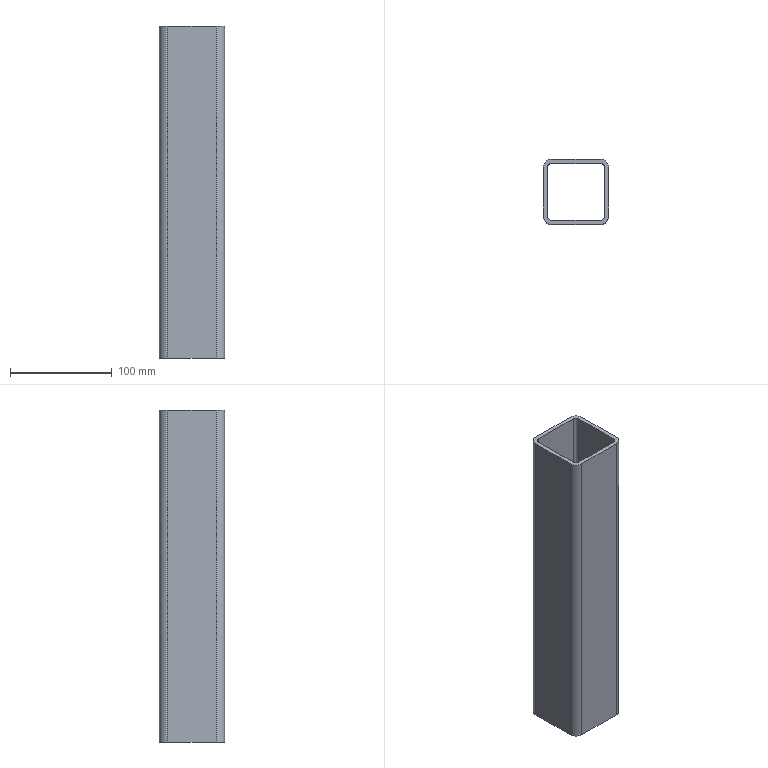Part | SolidWorks | features Extrusion 1 | 1 solid | 18 faces | box 64 x 64 x 326 mm | volume 299528 mm3 | plane 10 | cylinder 8 | commonest cylinder face diameters 8 x4 16 x4
STEP:
#1=CARTESIAN_POINT('',(-24.,32.,163.));
#2=VERTEX_POINT('',#1);
#3=CARTESIAN_POINT('',(-32.,24.,163.));
#4=VERTEX_POINT('',#3);
#5=CARTESIAN_POINT('',(-24.,24.,163.));
#6=DIRECTION('',(0.,0.,1.));
#7=DIRECTION('',(1.,0.,0.));
#8=AXIS2_PLACEMENT_3D('',#5,#6,#7);
#9=CIRCLE('',#8,8.);
#10=EDGE_CURVE('',#2,#4,#9,.T.);
#11=ORIENTED_EDGE('',*,*,#10,.T.);
#12=CARTESIAN_POINT('',(-32.,-24.,163.));
#13=VERTEX_POINT('',#12);
#14=CARTESIAN_POINT('',(-32.,24.,163.));
#15=DIRECTION('',(0.,-1.,0.));
#16=VECTOR('',#15,1000.);
#17=LINE('',#14,#16);
#18=EDGE_CURVE('',#4,#13,#17,.T.);
#19=ORIENTED_EDGE('',*,*,#18,.T.);
#20=CARTESIAN_POINT('',(-24.,-32.,163.));
#21=VERTEX_POINT('',#20);
#22=CARTESIAN_POINT('',(-24.,-24.,163.));
#23=DIRECTION('',(0.,0.,1.));
#24=DIRECTION('',(-1.,0.,0.));
#25=AXIS2_PLACEMENT_3D('',#22,#23,#24);
#26=CIRCLE('',#25,8.);
#27=EDGE_CURVE('',#13,#21,#26,.T.);
#28=ORIENTED_EDGE('',*,*,#27,.T.);
#29=CARTESIAN_POINT('',(24.,-32.,163.));
#30=VERTEX_POINT('',#29);
#31=CARTESIAN_POINT('',(24.,-32.,163.));
#32=DIRECTION('',(1.,0.,0.));
#33=VECTOR('',#32,1000.);
#34=LINE('',#31,#33);
#35=EDGE_CURVE('',#21,#30,#34,.T.);
#36=ORIENTED_EDGE('',*,*,#35,.T.);
#37=CARTESIAN_POINT('',(32.,-24.,163.));
#38=VERTEX_POINT('',#37);
#39=CARTESIAN_POINT('',(24.,-24.,163.));
#40=DIRECTION('',(0.,0.,1.));
#41=DIRECTION('',(1.,0.,0.));
#42=AXIS2_PLACEMENT_3D('',#39,#40,#41);
#43=CIRCLE('',#42,8.);
#44=EDGE_CURVE('',#30,#38,#43,.T.);
#45=ORIENTED_EDGE('',*,*,#44,.T.);
#46=CARTESIAN_POINT('',(32.,24.,163.));
#47=VERTEX_POINT('',#46);
#48=CARTESIAN_POINT('',(32.,-24.,163.));
#49=DIRECTION('',(0.,1.,0.));
#50=VECTOR('',#49,1000.);
#51=LINE('',#48,#50);
#52=EDGE_CURVE('',#38,#47,#51,.T.);
#53=ORIENTED_EDGE('',*,*,#52,.T.);
#54=CARTESIAN_POINT('',(24.,32.,163.));
#55=VERTEX_POINT('',#54);
#56=CARTESIAN_POINT('',(24.,24.,163.));
#57=DIRECTION('',(0.,0.,1.));
#58=DIRECTION('',(-1.,0.,0.));
#59=AXIS2_PLACEMENT_3D('',#56,#57,#58);
#60=CIRCLE('',#59,8.);
#61=EDGE_CURVE('',#47,#55,#60,.T.);
#62=ORIENTED_EDGE('',*,*,#61,.T.);
#63=CARTESIAN_POINT('',(0.,32.,163.));
#64=DIRECTION('',(-1.,0.,0.));
#65=VECTOR('',#64,1000.);
#66=LINE('',#63,#65);
#67=EDGE_CURVE('',#55,#2,#66,.T.);
#68=ORIENTED_EDGE('',*,*,#67,.T.);
#69=EDGE_LOOP('',(#11,#19,#28,#36,#45,#53,#62,#68));
#70=FACE_OUTER_BOUND('',#69,.T.);
#71=CARTESIAN_POINT('',(-28.,24.,163.));
#72=VERTEX_POINT('',#71);
#73=CARTESIAN_POINT('',(-28.,-24.,163.));
#74=VERTEX_POINT('',#73);
#75=CARTESIAN_POINT('',(-28.,24.,163.));
#76=DIRECTION('',(0.,-1.,0.));
#77=VECTOR('',#76,1000.);
#78=LINE('',#75,#77);
#79=EDGE_CURVE('',#72,#74,#78,.T.);
#80=ORIENTED_EDGE('',*,*,#79,.F.);
#81=CARTESIAN_POINT('',(-24.,28.,163.));
#82=VERTEX_POINT('',#81);
#83=CARTESIAN_POINT('',(-24.,24.,163.));
#84=DIRECTION('',(0.,0.,1.));
#85=DIRECTION('',(1.,0.,0.));
#86=AXIS2_PLACEMENT_3D('',#83,#84,#85);
#87=CIRCLE('',#86,4.);
#88=EDGE_CURVE('',#82,#72,#87,.T.);
#89=ORIENTED_EDGE('',*,*,#88,.F.);
#90=CARTESIAN_POINT('',(24.,28.,163.));
#91=VERTEX_POINT('',#90);
#92=CARTESIAN_POINT('',(0.,28.,163.));
#93=DIRECTION('',(-1.,0.,0.));
#94=VECTOR('',#93,1000.);
#95=LINE('',#92,#94);
#96=EDGE_CURVE('',#91,#82,#95,.T.);
#97=ORIENTED_EDGE('',*,*,#96,.F.);
#98=CARTESIAN_POINT('',(28.,24.,163.));
#99=VERTEX_POINT('',#98);
#100=CARTESIAN_POINT('',(24.,24.,163.));
#101=DIRECTION('',(0.,0.,1.));
#102=DIRECTION('',(-1.,0.,0.));
#103=AXIS2_PLACEMENT_3D('',#100,#101,#102);
#104=CIRCLE('',#103,4.);
#105=EDGE_CURVE('',#99,#91,#104,.T.);
#106=ORIENTED_EDGE('',*,*,#105,.F.);
#107=CARTESIAN_POINT('',(28.,-24.,163.));
#108=VERTEX_POINT('',#107);
#109=CARTESIAN_POINT('',(28.,-24.,163.));
#110=DIRECTION('',(0.,1.,0.));
#111=VECTOR('',#110,1000.);
#112=LINE('',#109,#111);
#113=EDGE_CURVE('',#108,#99,#112,.T.);
#114=ORIENTED_EDGE('',*,*,#113,.F.);
#115=CARTESIAN_POINT('',(24.,-28.,163.));
#116=VERTEX_POINT('',#115);
#117=CARTESIAN_POINT('',(24.,-24.,163.));
#118=DIRECTION('',(0.,0.,1.));
#119=DIRECTION('',(1.,0.,0.));
#120=AXIS2_PLACEMENT_3D('',#117,#118,#119);
#121=CIRCLE('',#120,4.);
#122=EDGE_CURVE('',#116,#108,#121,.T.);
#123=ORIENTED_EDGE('',*,*,#122,.F.);
#124=CARTESIAN_POINT('',(-24.,-28.,163.));
#125=VERTEX_POINT('',#124);
#126=CARTESIAN_POINT('',(24.,-28.,163.));
#127=DIRECTION('',(1.,0.,0.));
#128=VECTOR('',#127,1000.);
#129=LINE('',#126,#128);
#130=EDGE_CURVE('',#125,#116,#129,.T.);
#131=ORIENTED_EDGE('',*,*,#130,.F.);
#132=CARTESIAN_POINT('',(-24.,-24.,163.));
#133=DIRECTION('',(0.,0.,1.));
#134=DIRECTION('',(-1.,0.,0.));
#135=AXIS2_PLACEMENT_3D('',#132,#133,#134);
#136=CIRCLE('',#135,4.);
#137=EDGE_CURVE('',#74,#125,#136,.T.);
#138=ORIENTED_EDGE('',*,*,#137,.F.);
#139=EDGE_LOOP('',(#80,#89,#97,#106,#114,#123,#131,#138));
#140=FACE_BOUND('',#139,.T.);
#141=CARTESIAN_POINT('',(-24.,24.,163.));
#142=DIRECTION('',(0.,0.,1.));
#143=DIRECTION('',(1.,0.,0.));
#144=AXIS2_PLACEMENT_3D('',#141,#142,#143);
#145=PLANE('',#144);
#146=ADVANCED_FACE('',(#70,#140),#145,.T.);
#147=CARTESIAN_POINT('',(-24.,32.,-163.));
#148=VERTEX_POINT('',#147);
#149=CARTESIAN_POINT('',(-32.,24.,-163.));
#150=VERTEX_POINT('',#149);
#151=CARTESIAN_POINT('',(-24.,24.,-163.));
#152=DIRECTION('',(0.,0.,1.));
#153=DIRECTION('',(1.,0.,0.));
#154=AXIS2_PLACEMENT_3D('',#151,#152,#153);
#155=CIRCLE('',#154,8.);
#156=EDGE_CURVE('',#148,#150,#155,.T.);
#157=ORIENTED_EDGE('',*,*,#156,.F.);
#158=CARTESIAN_POINT('',(24.,32.,-163.));
#159=VERTEX_POINT('',#158);
#160=CARTESIAN_POINT('',(0.,32.,-163.));
#161=DIRECTION('',(-1.,0.,0.));
#162=VECTOR('',#161,1000.);
#163=LINE('',#160,#162);
#164=EDGE_CURVE('',#159,#148,#163,.T.);
#165=ORIENTED_EDGE('',*,*,#164,.F.);
#166=CARTESIAN_POINT('',(32.,24.,-163.));
#167=VERTEX_POINT('',#166);
#168=CARTESIAN_POINT('',(24.,24.,-163.));
#169=DIRECTION('',(0.,0.,1.));
#170=DIRECTION('',(-1.,0.,0.));
#171=AXIS2_PLACEMENT_3D('',#168,#169,#170);
#172=CIRCLE('',#171,8.);
#173=EDGE_CURVE('',#167,#159,#172,.T.);
#174=ORIENTED_EDGE('',*,*,#173,.F.);
#175=CARTESIAN_POINT('',(32.,-24.,-163.));
#176=VERTEX_POINT('',#175);
#177=CARTESIAN_POINT('',(32.,24.,-163.));
#178=DIRECTION('',(0.,1.,0.));
#179=VECTOR('',#178,1000.);
#180=LINE('',#177,#179);
#181=EDGE_CURVE('',#176,#167,#180,.T.);
#182=ORIENTED_EDGE('',*,*,#181,.F.);
#183=CARTESIAN_POINT('',(24.,-32.,-163.));
#184=VERTEX_POINT('',#183);
#185=CARTESIAN_POINT('',(24.,-24.,-163.));
#186=DIRECTION('',(0.,0.,1.));
#187=DIRECTION('',(1.,0.,0.));
#188=AXIS2_PLACEMENT_3D('',#185,#186,#187);
#189=CIRCLE('',#188,8.);
#190=EDGE_CURVE('',#184,#176,#189,.T.);
#191=ORIENTED_EDGE('',*,*,#190,.F.);
#192=CARTESIAN_POINT('',(-24.,-32.,-163.));
#193=VERTEX_POINT('',#192);
#194=CARTESIAN_POINT('',(24.,-32.,-163.));
#195=DIRECTION('',(1.,0.,0.));
#196=VECTOR('',#195,1000.);
#197=LINE('',#194,#196);
#198=EDGE_CURVE('',#193,#184,#197,.T.);
#199=ORIENTED_EDGE('',*,*,#198,.F.);
#200=CARTESIAN_POINT('',(-32.,-24.,-163.));
#201=VERTEX_POINT('',#200);
#202=CARTESIAN_POINT('',(-24.,-24.,-163.));
#203=DIRECTION('',(0.,0.,1.));
#204=DIRECTION('',(-1.,0.,0.));
#205=AXIS2_PLACEMENT_3D('',#202,#203,#204);
#206=CIRCLE('',#205,8.);
#207=EDGE_CURVE('',#201,#193,#206,.T.);
#208=ORIENTED_EDGE('',*,*,#207,.F.);
#209=CARTESIAN_POINT('',(-32.,-24.,-163.));
#210=DIRECTION('',(0.,-1.,0.));
#211=VECTOR('',#210,1000.);
#212=LINE('',#209,#211);
#213=EDGE_CURVE('',#150,#201,#212,.T.);
#214=ORIENTED_EDGE('',*,*,#213,.F.);
#215=EDGE_LOOP('',(#157,#165,#174,#182,#191,#199,#208,#214));
#216=FACE_OUTER_BOUND('',#215,.T.);
#217=CARTESIAN_POINT('',(-24.,28.,-163.));
#218=VERTEX_POINT('',#217);
#219=CARTESIAN_POINT('',(-28.,24.,-163.));
#220=VERTEX_POINT('',#219);
#221=CARTESIAN_POINT('',(-24.,24.,-163.));
#222=DIRECTION('',(0.,0.,1.));
#223=DIRECTION('',(1.,0.,0.));
#224=AXIS2_PLACEMENT_3D('',#221,#222,#223);
#225=CIRCLE('',#224,4.);
#226=EDGE_CURVE('',#218,#220,#225,.T.);
#227=ORIENTED_EDGE('',*,*,#226,.T.);
#228=CARTESIAN_POINT('',(-28.,-24.,-163.));
#229=VERTEX_POINT('',#228);
#230=CARTESIAN_POINT('',(-28.,-24.,-163.));
#231=DIRECTION('',(0.,-1.,0.));
#232=VECTOR('',#231,1000.);
#233=LINE('',#230,#232);
#234=EDGE_CURVE('',#220,#229,#233,.T.);
#235=ORIENTED_EDGE('',*,*,#234,.T.);
#236=CARTESIAN_POINT('',(-24.,-28.,-163.));
#237=VERTEX_POINT('',#236);
#238=CARTESIAN_POINT('',(-24.,-24.,-163.));
#239=DIRECTION('',(0.,0.,1.));
#240=DIRECTION('',(-1.,0.,0.));
#241=AXIS2_PLACEMENT_3D('',#238,#239,#240);
#242=CIRCLE('',#241,4.);
#243=EDGE_CURVE('',#229,#237,#242,.T.);
#244=ORIENTED_EDGE('',*,*,#243,.T.);
#245=CARTESIAN_POINT('',(24.,-28.,-163.));
#246=VERTEX_POINT('',#245);
#247=CARTESIAN_POINT('',(24.,-28.,-163.));
#248=DIRECTION('',(1.,0.,0.));
#249=VECTOR('',#248,1000.);
#250=LINE('',#247,#249);
#251=EDGE_CURVE('',#237,#246,#250,.T.);
#252=ORIENTED_EDGE('',*,*,#251,.T.);
#253=CARTESIAN_POINT('',(28.,-24.,-163.));
#254=VERTEX_POINT('',#253);
#255=CARTESIAN_POINT('',(24.,-24.,-163.));
#256=DIRECTION('',(0.,0.,1.));
#257=DIRECTION('',(1.,0.,0.));
#258=AXIS2_PLACEMENT_3D('',#255,#256,#257);
#259=CIRCLE('',#258,4.);
#260=EDGE_CURVE('',#246,#254,#259,.T.);
#261=ORIENTED_EDGE('',*,*,#260,.T.);
#262=CARTESIAN_POINT('',(28.,24.,-163.));
#263=VERTEX_POINT('',#262);
#264=CARTESIAN_POINT('',(28.,24.,-163.));
#265=DIRECTION('',(0.,1.,0.));
#266=VECTOR('',#265,1000.);
#267=LINE('',#264,#266);
#268=EDGE_CURVE('',#254,#263,#267,.T.);
#269=ORIENTED_EDGE('',*,*,#268,.T.);
#270=CARTESIAN_POINT('',(24.,28.,-163.));
#271=VERTEX_POINT('',#270);
#272=CARTESIAN_POINT('',(24.,24.,-163.));
#273=DIRECTION('',(0.,0.,1.));
#274=DIRECTION('',(-1.,0.,0.));
#275=AXIS2_PLACEMENT_3D('',#272,#273,#274);
#276=CIRCLE('',#275,4.);
#277=EDGE_CURVE('',#263,#271,#276,.T.);
#278=ORIENTED_EDGE('',*,*,#277,.T.);
#279=CARTESIAN_POINT('',(0.,28.,-163.));
#280=DIRECTION('',(-1.,0.,0.));
#281=VECTOR('',#280,1000.);
#282=LINE('',#279,#281);
#283=EDGE_CURVE('',#271,#218,#282,.T.);
#284=ORIENTED_EDGE('',*,*,#283,.T.);
#285=EDGE_LOOP('',(#227,#235,#244,#252,#261,#269,#278,#284));
#286=FACE_BOUND('',#285,.T.);
#287=CARTESIAN_POINT('',(-24.,24.,-163.));
#288=DIRECTION('',(0.,0.,1.));
#289=DIRECTION('',(1.,0.,0.));
#290=AXIS2_PLACEMENT_3D('',#287,#288,#289);
#291=PLANE('',#290);
#292=ADVANCED_FACE('',(#216,#286),#291,.F.);
#293=ORIENTED_EDGE('',*,*,#156,.T.);
#294=CARTESIAN_POINT('',(-32.,24.,163.));
#295=DIRECTION('',(0.,0.,-1.));
#296=VECTOR('',#295,1000.);
#297=LINE('',#294,#296);
#298=EDGE_CURVE('',#4,#150,#297,.T.);
#299=ORIENTED_EDGE('',*,*,#298,.F.);
#300=ORIENTED_EDGE('',*,*,#10,.F.);
#301=CARTESIAN_POINT('',(-24.,32.,163.));
#302=DIRECTION('',(0.,0.,-1.));
#303=VECTOR('',#302,1000.);
#304=LINE('',#301,#303);
#305=EDGE_CURVE('',#2,#148,#304,.T.);
#306=ORIENTED_EDGE('',*,*,#305,.T.);
#307=EDGE_LOOP('',(#293,#299,#300,#306));
#308=FACE_OUTER_BOUND('',#307,.T.);
#309=CARTESIAN_POINT('',(-24.,24.,163.));
#310=DIRECTION('',(0.,0.,-1.));
#311=DIRECTION('',(-1.,0.,0.));
#312=AXIS2_PLACEMENT_3D('',#309,#310,#311);
#313=CYLINDRICAL_SURFACE('',#312,8.);
#314=ADVANCED_FACE('',(#308),#313,.T.);
#315=ORIENTED_EDGE('',*,*,#213,.T.);
#316=CARTESIAN_POINT('',(-32.,-24.,163.));
#317=DIRECTION('',(0.,0.,-1.));
#318=VECTOR('',#317,1000.);
#319=LINE('',#316,#318);
#320=EDGE_CURVE('',#13,#201,#319,.T.);
#321=ORIENTED_EDGE('',*,*,#320,.F.);
#322=ORIENTED_EDGE('',*,*,#18,.F.);
#323=ORIENTED_EDGE('',*,*,#298,.T.);
#324=EDGE_LOOP('',(#315,#321,#322,#323));
#325=FACE_OUTER_BOUND('',#324,.T.);
#326=CARTESIAN_POINT('',(-32.,-24.,163.));
#327=DIRECTION('',(1.,0.,0.));
#328=DIRECTION('',(0.,0.,-1.));
#329=AXIS2_PLACEMENT_3D('',#326,#327,#328);
#330=PLANE('',#329);
#331=ADVANCED_FACE('',(#325),#330,.F.);
#332=ORIENTED_EDGE('',*,*,#207,.T.);
#333=CARTESIAN_POINT('',(-24.,-32.,163.));
#334=DIRECTION('',(0.,0.,-1.));
#335=VECTOR('',#334,1000.);
#336=LINE('',#333,#335);
#337=EDGE_CURVE('',#21,#193,#336,.T.);
#338=ORIENTED_EDGE('',*,*,#337,.F.);
#339=ORIENTED_EDGE('',*,*,#27,.F.);
#340=ORIENTED_EDGE('',*,*,#320,.T.);
#341=EDGE_LOOP('',(#332,#338,#339,#340));
#342=FACE_OUTER_BOUND('',#341,.T.);
#343=CARTESIAN_POINT('',(-24.,-24.,163.));
#344=DIRECTION('',(0.,0.,-1.));
#345=DIRECTION('',(-1.,0.,0.));
#346=AXIS2_PLACEMENT_3D('',#343,#344,#345);
#347=CYLINDRICAL_SURFACE('',#346,8.);
#348=ADVANCED_FACE('',(#342),#347,.T.);
#349=ORIENTED_EDGE('',*,*,#198,.T.);
#350=CARTESIAN_POINT('',(24.,-32.,163.));
#351=DIRECTION('',(0.,0.,-1.));
#352=VECTOR('',#351,1000.);
#353=LINE('',#350,#352);
#354=EDGE_CURVE('',#30,#184,#353,.T.);
#355=ORIENTED_EDGE('',*,*,#354,.F.);
#356=ORIENTED_EDGE('',*,*,#35,.F.);
#357=ORIENTED_EDGE('',*,*,#337,.T.);
#358=EDGE_LOOP('',(#349,#355,#356,#357));
#359=FACE_OUTER_BOUND('',#358,.T.);
#360=CARTESIAN_POINT('',(24.,-32.,163.));
#361=DIRECTION('',(0.,1.,0.));
#362=DIRECTION('',(-1.,0.,0.));
#363=AXIS2_PLACEMENT_3D('',#360,#361,#362);
#364=PLANE('',#363);
#365=ADVANCED_FACE('',(#359),#364,.F.);
#366=ORIENTED_EDGE('',*,*,#190,.T.);
#367=CARTESIAN_POINT('',(32.,-24.,163.));
#368=DIRECTION('',(0.,0.,-1.));
#369=VECTOR('',#368,1000.);
#370=LINE('',#367,#369);
#371=EDGE_CURVE('',#38,#176,#370,.T.);
#372=ORIENTED_EDGE('',*,*,#371,.F.);
#373=ORIENTED_EDGE('',*,*,#44,.F.);
#374=ORIENTED_EDGE('',*,*,#354,.T.);
#375=EDGE_LOOP('',(#366,#372,#373,#374));
#376=FACE_OUTER_BOUND('',#375,.T.);
#377=CARTESIAN_POINT('',(24.,-24.,163.));
#378=DIRECTION('',(0.,0.,-1.));
#379=DIRECTION('',(-1.,0.,0.));
#380=AXIS2_PLACEMENT_3D('',#377,#378,#379);
#381=CYLINDRICAL_SURFACE('',#380,8.);
#382=ADVANCED_FACE('',(#376),#381,.T.);
#383=ORIENTED_EDGE('',*,*,#181,.T.);
#384=CARTESIAN_POINT('',(32.,24.,163.));
#385=DIRECTION('',(0.,0.,-1.));
#386=VECTOR('',#385,1000.);
#387=LINE('',#384,#386);
#388=EDGE_CURVE('',#47,#167,#387,.T.);
#389=ORIENTED_EDGE('',*,*,#388,.F.);
#390=ORIENTED_EDGE('',*,*,#52,.F.);
#391=ORIENTED_EDGE('',*,*,#371,.T.);
#392=EDGE_LOOP('',(#383,#389,#390,#391));
#393=FACE_OUTER_BOUND('',#392,.T.);
#394=CARTESIAN_POINT('',(32.,24.,163.));
#395=DIRECTION('',(-1.,0.,0.));
#396=DIRECTION('',(0.,0.,1.));
#397=AXIS2_PLACEMENT_3D('',#394,#395,#396);
#398=PLANE('',#397);
#399=ADVANCED_FACE('',(#393),#398,.F.);
#400=ORIENTED_EDGE('',*,*,#173,.T.);
#401=CARTESIAN_POINT('',(24.,32.,163.));
#402=DIRECTION('',(0.,0.,-1.));
#403=VECTOR('',#402,1000.);
#404=LINE('',#401,#403);
#405=EDGE_CURVE('',#55,#159,#404,.T.);
#406=ORIENTED_EDGE('',*,*,#405,.F.);
#407=ORIENTED_EDGE('',*,*,#61,.F.);
#408=ORIENTED_EDGE('',*,*,#388,.T.);
#409=EDGE_LOOP('',(#400,#406,#407,#408));
#410=FACE_OUTER_BOUND('',#409,.T.);
#411=CARTESIAN_POINT('',(24.,24.,163.));
#412=DIRECTION('',(0.,0.,-1.));
#413=DIRECTION('',(-1.,0.,0.));
#414=AXIS2_PLACEMENT_3D('',#411,#412,#413);
#415=CYLINDRICAL_SURFACE('',#414,8.);
#416=ADVANCED_FACE('',(#410),#415,.T.);
#417=ORIENTED_EDGE('',*,*,#164,.T.);
#418=ORIENTED_EDGE('',*,*,#305,.F.);
#419=ORIENTED_EDGE('',*,*,#67,.F.);
#420=ORIENTED_EDGE('',*,*,#405,.T.);
#421=EDGE_LOOP('',(#417,#418,#419,#420));
#422=FACE_OUTER_BOUND('',#421,.T.);
#423=CARTESIAN_POINT('',(0.,32.,163.));
#424=DIRECTION('',(0.,-1.,0.));
#425=DIRECTION('',(0.,0.,-1.));
#426=AXIS2_PLACEMENT_3D('',#423,#424,#425);
#427=PLANE('',#426);
#428=ADVANCED_FACE('',(#422),#427,.F.);
#429=ORIENTED_EDGE('',*,*,#226,.F.);
#430=CARTESIAN_POINT('',(-24.,28.,163.));
#431=DIRECTION('',(0.,0.,-1.));
#432=VECTOR('',#431,1000.);
#433=LINE('',#430,#432);
#434=EDGE_CURVE('',#82,#218,#433,.T.);
#435=ORIENTED_EDGE('',*,*,#434,.F.);
#436=ORIENTED_EDGE('',*,*,#88,.T.);
#437=CARTESIAN_POINT('',(-28.,24.,163.));
#438=DIRECTION('',(0.,0.,-1.));
#439=VECTOR('',#438,1000.);
#440=LINE('',#437,#439);
#441=EDGE_CURVE('',#72,#220,#440,.T.);
#442=ORIENTED_EDGE('',*,*,#441,.T.);
#443=EDGE_LOOP('',(#429,#435,#436,#442));
#444=FACE_OUTER_BOUND('',#443,.T.);
#445=CARTESIAN_POINT('',(-24.,24.,163.));
#446=DIRECTION('',(0.,0.,-1.));
#447=DIRECTION('',(-1.,0.,0.));
#448=AXIS2_PLACEMENT_3D('',#445,#446,#447);
#449=CYLINDRICAL_SURFACE('',#448,4.);
#450=ADVANCED_FACE('',(#444),#449,.F.);
#451=ORIENTED_EDGE('',*,*,#234,.F.);
#452=ORIENTED_EDGE('',*,*,#441,.F.);
#453=ORIENTED_EDGE('',*,*,#79,.T.);
#454=CARTESIAN_POINT('',(-28.,-24.,163.));
#455=DIRECTION('',(0.,0.,-1.));
#456=VECTOR('',#455,1000.);
#457=LINE('',#454,#456);
#458=EDGE_CURVE('',#74,#229,#457,.T.);
#459=ORIENTED_EDGE('',*,*,#458,.T.);
#460=EDGE_LOOP('',(#451,#452,#453,#459));
#461=FACE_OUTER_BOUND('',#460,.T.);
#462=CARTESIAN_POINT('',(-28.,-24.,163.));
#463=DIRECTION('',(1.,0.,0.));
#464=DIRECTION('',(0.,1.,0.));
#465=AXIS2_PLACEMENT_3D('',#462,#463,#464);
#466=PLANE('',#465);
#467=ADVANCED_FACE('',(#461),#466,.T.);
#468=ORIENTED_EDGE('',*,*,#243,.F.);
#469=ORIENTED_EDGE('',*,*,#458,.F.);
#470=ORIENTED_EDGE('',*,*,#137,.T.);
#471=CARTESIAN_POINT('',(-24.,-28.,163.));
#472=DIRECTION('',(0.,0.,-1.));
#473=VECTOR('',#472,1000.);
#474=LINE('',#471,#473);
#475=EDGE_CURVE('',#125,#237,#474,.T.);
#476=ORIENTED_EDGE('',*,*,#475,.T.);
#477=EDGE_LOOP('',(#468,#469,#470,#476));
#478=FACE_OUTER_BOUND('',#477,.T.);
#479=CARTESIAN_POINT('',(-24.,-24.,163.));
#480=DIRECTION('',(0.,0.,-1.));
#481=DIRECTION('',(-1.,0.,0.));
#482=AXIS2_PLACEMENT_3D('',#479,#480,#481);
#483=CYLINDRICAL_SURFACE('',#482,4.);
#484=ADVANCED_FACE('',(#478),#483,.F.);
#485=ORIENTED_EDGE('',*,*,#251,.F.);
#486=ORIENTED_EDGE('',*,*,#475,.F.);
#487=ORIENTED_EDGE('',*,*,#130,.T.);
#488=CARTESIAN_POINT('',(24.,-28.,163.));
#489=DIRECTION('',(0.,0.,-1.));
#490=VECTOR('',#489,1000.);
#491=LINE('',#488,#490);
#492=EDGE_CURVE('',#116,#246,#491,.T.);
#493=ORIENTED_EDGE('',*,*,#492,.T.);
#494=EDGE_LOOP('',(#485,#486,#487,#493));
#495=FACE_OUTER_BOUND('',#494,.T.);
#496=CARTESIAN_POINT('',(24.,-28.,163.));
#497=DIRECTION('',(0.,1.,0.));
#498=DIRECTION('',(-1.,0.,0.));
#499=AXIS2_PLACEMENT_3D('',#496,#497,#498);
#500=PLANE('',#499);
#501=ADVANCED_FACE('',(#495),#500,.T.);
#502=ORIENTED_EDGE('',*,*,#260,.F.);
#503=ORIENTED_EDGE('',*,*,#492,.F.);
#504=ORIENTED_EDGE('',*,*,#122,.T.);
#505=CARTESIAN_POINT('',(28.,-24.,163.));
#506=DIRECTION('',(0.,0.,-1.));
#507=VECTOR('',#506,1000.);
#508=LINE('',#505,#507);
#509=EDGE_CURVE('',#108,#254,#508,.T.);
#510=ORIENTED_EDGE('',*,*,#509,.T.);
#511=EDGE_LOOP('',(#502,#503,#504,#510));
#512=FACE_OUTER_BOUND('',#511,.T.);
#513=CARTESIAN_POINT('',(24.,-24.,163.));
#514=DIRECTION('',(0.,0.,-1.));
#515=DIRECTION('',(-1.,0.,0.));
#516=AXIS2_PLACEMENT_3D('',#513,#514,#515);
#517=CYLINDRICAL_SURFACE('',#516,4.);
#518=ADVANCED_FACE('',(#512),#517,.F.);
#519=ORIENTED_EDGE('',*,*,#268,.F.);
#520=ORIENTED_EDGE('',*,*,#509,.F.);
#521=ORIENTED_EDGE('',*,*,#113,.T.);
#522=CARTESIAN_POINT('',(28.,24.,163.));
#523=DIRECTION('',(0.,0.,-1.));
#524=VECTOR('',#523,1000.);
#525=LINE('',#522,#524);
#526=EDGE_CURVE('',#99,#263,#525,.T.);
#527=ORIENTED_EDGE('',*,*,#526,.T.);
#528=EDGE_LOOP('',(#519,#520,#521,#527));
#529=FACE_OUTER_BOUND('',#528,.T.);
#530=CARTESIAN_POINT('',(28.,24.,163.));
#531=DIRECTION('',(-1.,0.,0.));
#532=DIRECTION('',(0.,-1.,0.));
#533=AXIS2_PLACEMENT_3D('',#530,#531,#532);
#534=PLANE('',#533);
#535=ADVANCED_FACE('',(#529),#534,.T.);
#536=ORIENTED_EDGE('',*,*,#277,.F.);
#537=ORIENTED_EDGE('',*,*,#526,.F.);
#538=ORIENTED_EDGE('',*,*,#105,.T.);
#539=CARTESIAN_POINT('',(24.,28.,163.));
#540=DIRECTION('',(0.,0.,-1.));
#541=VECTOR('',#540,1000.);
#542=LINE('',#539,#541);
#543=EDGE_CURVE('',#91,#271,#542,.T.);
#544=ORIENTED_EDGE('',*,*,#543,.T.);
#545=EDGE_LOOP('',(#536,#537,#538,#544));
#546=FACE_OUTER_BOUND('',#545,.T.);
#547=CARTESIAN_POINT('',(24.,24.,163.));
#548=DIRECTION('',(0.,0.,-1.));
#549=DIRECTION('',(-1.,0.,0.));
#550=AXIS2_PLACEMENT_3D('',#547,#548,#549);
#551=CYLINDRICAL_SURFACE('',#550,4.);
#552=ADVANCED_FACE('',(#546),#551,.F.);
#553=ORIENTED_EDGE('',*,*,#283,.F.);
#554=ORIENTED_EDGE('',*,*,#543,.F.);
#555=ORIENTED_EDGE('',*,*,#96,.T.);
#556=ORIENTED_EDGE('',*,*,#434,.T.);
#557=EDGE_LOOP('',(#553,#554,#555,#556));
#558=FACE_OUTER_BOUND('',#557,.T.);
#559=CARTESIAN_POINT('',(0.,28.,163.));
#560=DIRECTION('',(0.,-1.,0.));
#561=DIRECTION('',(0.,0.,-1.));
#562=AXIS2_PLACEMENT_3D('',#559,#560,#561);
#563=PLANE('',#562);
#564=ADVANCED_FACE('',(#558),#563,.T.);
#565=CLOSED_SHELL('',(#146,#292,#314,#331,#348,#365,#382,#399,#416,#428,#450,#467,#484,#501,#518,#535,#552,#564));
#566=MANIFOLD_SOLID_BREP('',#565);
#567=CARTESIAN_POINT('',(0.,0.,0.));
#568=DIRECTION('',(0.,0.,1.));
#569=DIRECTION('',(1.,0.,0.));
#570=AXIS2_PLACEMENT_3D('',#567,#568,#569);
#571=(LENGTH_UNIT()NAMED_UNIT(*)SI_UNIT(.MILLI.,.METRE.));
#572=UNCERTAINTY_MEASURE_WITH_UNIT(LENGTH_MEASURE(0.00001),#571,'','');
#573=(NAMED_UNIT(*)PLANE_ANGLE_UNIT()SI_UNIT($,.RADIAN.));
#574=(NAMED_UNIT(*)SI_UNIT($,.STERADIAN.)SOLID_ANGLE_UNIT());
#575=(GEOMETRIC_REPRESENTATION_CONTEXT(3)GLOBAL_UNCERTAINTY_ASSIGNED_CONTEXT((#572))GLOBAL_UNIT_ASSIGNED_CONTEXT((#571,#573,#574))REPRESENTATION_CONTEXT('',''));
#576=ADVANCED_BREP_SHAPE_REPRESENTATION('',(#566,#570),#575);